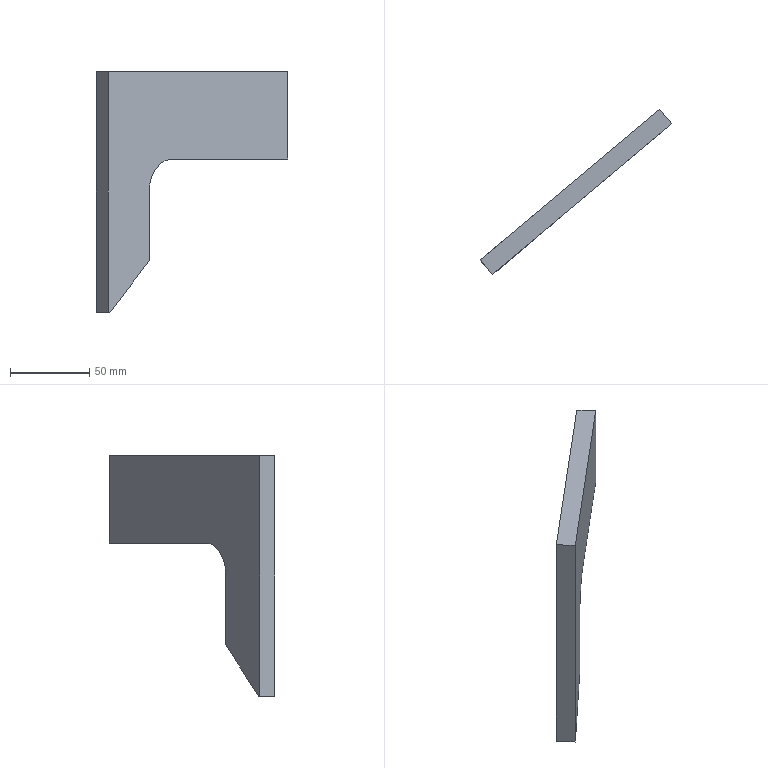Part | NX | features solid 2 | 1 solid | 10 faces | box 121.088 x 104.325 x 152 mm | volume 131882 mm3 | plane 9 | cylinder 1 | commonest cylinder face diameters 40 x1
STEP:
#1=CARTESIAN_POINT('',(765.225,419.33,-5.145));
#2=VERTEX_POINT('',#1);
#3=CARTESIAN_POINT('',(751.743,408.018,-25.));
#4=VERTEX_POINT('',#3);
#5=CARTESIAN_POINT('',(767.064,420.874,-25.));
#6=DIRECTION('',(0.6428,-0.766,0.));
#7=DIRECTION('',(0.766,0.6428,0.));
#8=AXIS2_PLACEMENT_3D('',#5,#6,#7);
#9=CIRCLE('',#8,20.);
#10=EDGE_CURVE('',#2,#4,#9,.T.);
#11=ORIENTED_EDGE('',*,*,#10,.F.);
#12=CARTESIAN_POINT('',(772.938,410.138,-5.145));
#13=VERTEX_POINT('',#12);
#14=CARTESIAN_POINT('',(772.938,410.138,-5.145));
#15=DIRECTION('',(-0.6428,0.766,0.));
#16=VECTOR('',#15,1000.);
#17=LINE('',#14,#16);
#18=EDGE_CURVE('',#13,#2,#17,.T.);
#19=ORIENTED_EDGE('',*,*,#18,.F.);
#20=CARTESIAN_POINT('',(759.457,398.826,-25.));
#21=VERTEX_POINT('',#20);
#22=CARTESIAN_POINT('',(774.777,411.681,-25.));
#23=DIRECTION('',(0.6428,-0.766,0.));
#24=DIRECTION('',(0.766,0.6428,0.));
#25=AXIS2_PLACEMENT_3D('',#22,#23,#24);
#26=CIRCLE('',#25,20.);
#27=EDGE_CURVE('',#13,#21,#26,.T.);
#28=ORIENTED_EDGE('',*,*,#27,.T.);
#29=CARTESIAN_POINT('',(759.457,398.826,-25.));
#30=DIRECTION('',(-0.6428,0.766,0.));
#31=VECTOR('',#30,1000.);
#32=LINE('',#29,#31);
#33=EDGE_CURVE('',#21,#4,#32,.T.);
#34=ORIENTED_EDGE('',*,*,#33,.T.);
#35=EDGE_LOOP('',(#11,#19,#28,#34));
#36=FACE_BOUND('',#35,.T.);
#37=CARTESIAN_POINT('',(774.777,411.681,-25.));
#38=DIRECTION('',(-0.6428,0.766,0.));
#39=DIRECTION('',(0.,0.,-1.));
#40=AXIS2_PLACEMENT_3D('',#37,#38,#39);
#41=CYLINDRICAL_SURFACE('',#40,20.);
#42=ADVANCED_FACE('',(#36),#41,.F.);
#43=CARTESIAN_POINT('',(839.225,481.424,-5.145));
#44=VERTEX_POINT('',#43);
#45=CARTESIAN_POINT('',(747.3,404.29,-5.145));
#46=DIRECTION('',(0.766,0.6428,0.));
#47=VECTOR('',#46,1000.);
#48=LINE('',#45,#47);
#49=EDGE_CURVE('',#2,#44,#48,.T.);
#50=ORIENTED_EDGE('',*,*,#49,.T.);
#51=CARTESIAN_POINT('',(846.939,472.232,-5.145));
#52=VERTEX_POINT('',#51);
#53=CARTESIAN_POINT('',(846.939,472.232,-5.145));
#54=DIRECTION('',(-0.6428,0.766,0.));
#55=VECTOR('',#54,1000.);
#56=LINE('',#53,#55);
#57=EDGE_CURVE('',#52,#44,#56,.T.);
#58=ORIENTED_EDGE('',*,*,#57,.F.);
#59=CARTESIAN_POINT('',(755.013,395.097,-5.145));
#60=DIRECTION('',(0.766,0.6428,0.));
#61=VECTOR('',#60,1000.);
#62=LINE('',#59,#61);
#63=EDGE_CURVE('',#13,#52,#62,.T.);
#64=ORIENTED_EDGE('',*,*,#63,.F.);
#65=ORIENTED_EDGE('',*,*,#18,.T.);
#66=EDGE_LOOP('',(#50,#58,#64,#65));
#67=FACE_BOUND('',#66,.T.);
#68=CARTESIAN_POINT('',(755.013,395.097,-5.145));
#69=DIRECTION('',(0.,0.,1.));
#70=DIRECTION('',(-0.766,-0.6428,0.));
#71=AXIS2_PLACEMENT_3D('',#68,#69,#70);
#72=PLANE('',#71);
#73=ADVANCED_FACE('',(#67),#72,.F.);
#74=CARTESIAN_POINT('',(839.225,481.424,50.));
#75=VERTEX_POINT('',#74);
#76=CARTESIAN_POINT('',(839.225,481.424,-5.145));
#77=DIRECTION('',(0.,0.,1.));
#78=VECTOR('',#77,1000.);
#79=LINE('',#76,#78);
#80=EDGE_CURVE('',#44,#75,#79,.T.);
#81=ORIENTED_EDGE('',*,*,#80,.T.);
#82=CARTESIAN_POINT('',(846.939,472.232,50.));
#83=VERTEX_POINT('',#82);
#84=CARTESIAN_POINT('',(846.939,472.232,50.));
#85=DIRECTION('',(-0.6428,0.766,0.));
#86=VECTOR('',#85,1000.);
#87=LINE('',#84,#86);
#88=EDGE_CURVE('',#83,#75,#87,.T.);
#89=ORIENTED_EDGE('',*,*,#88,.F.);
#90=CARTESIAN_POINT('',(846.939,472.232,-5.145));
#91=DIRECTION('',(0.,0.,1.));
#92=VECTOR('',#91,1000.);
#93=LINE('',#90,#92);
#94=EDGE_CURVE('',#52,#83,#93,.T.);
#95=ORIENTED_EDGE('',*,*,#94,.F.);
#96=ORIENTED_EDGE('',*,*,#57,.T.);
#97=EDGE_LOOP('',(#81,#89,#95,#96));
#98=FACE_BOUND('',#97,.T.);
#99=CARTESIAN_POINT('',(846.939,472.232,-5.145));
#100=DIRECTION('',(-0.766,-0.6428,0.));
#101=DIRECTION('',(0.,0.,-1.));
#102=AXIS2_PLACEMENT_3D('',#99,#100,#101);
#103=PLANE('',#102);
#104=ADVANCED_FACE('',(#98),#103,.F.);
#105=CARTESIAN_POINT('',(725.851,386.292,-102.));
#106=VERTEX_POINT('',#105);
#107=CARTESIAN_POINT('',(725.851,386.292,50.));
#108=VERTEX_POINT('',#107);
#109=CARTESIAN_POINT('',(725.851,386.292,-102.));
#110=DIRECTION('',(0.,0.,1.));
#111=VECTOR('',#110,1000.);
#112=LINE('',#109,#111);
#113=EDGE_CURVE('',#106,#108,#112,.T.);
#114=ORIENTED_EDGE('',*,*,#113,.F.);
#115=CARTESIAN_POINT('',(733.564,377.099,-102.));
#116=VERTEX_POINT('',#115);
#117=CARTESIAN_POINT('',(733.564,377.099,-102.));
#118=DIRECTION('',(-0.6428,0.766,0.));
#119=VECTOR('',#118,1000.);
#120=LINE('',#117,#119);
#121=EDGE_CURVE('',#116,#106,#120,.T.);
#122=ORIENTED_EDGE('',*,*,#121,.F.);
#123=CARTESIAN_POINT('',(733.564,377.099,50.));
#124=VERTEX_POINT('',#123);
#125=CARTESIAN_POINT('',(733.564,377.099,-102.));
#126=DIRECTION('',(0.,0.,1.));
#127=VECTOR('',#126,1000.);
#128=LINE('',#125,#127);
#129=EDGE_CURVE('',#116,#124,#128,.T.);
#130=ORIENTED_EDGE('',*,*,#129,.T.);
#131=CARTESIAN_POINT('',(733.564,377.099,50.));
#132=DIRECTION('',(-0.6428,0.766,0.));
#133=VECTOR('',#132,1000.);
#134=LINE('',#131,#133);
#135=EDGE_CURVE('',#124,#108,#134,.T.);
#136=ORIENTED_EDGE('',*,*,#135,.T.);
#137=EDGE_LOOP('',(#114,#122,#130,#136));
#138=FACE_BOUND('',#137,.T.);
#139=CARTESIAN_POINT('',(733.564,377.099,-102.));
#140=DIRECTION('',(-0.766,-0.6428,0.));
#141=DIRECTION('',(0.,0.,-1.));
#142=AXIS2_PLACEMENT_3D('',#139,#140,#141);
#143=PLANE('',#142);
#144=ADVANCED_FACE('',(#138),#143,.T.);
#145=CARTESIAN_POINT('',(726.847,387.128,-102.));
#146=VERTEX_POINT('',#145);
#147=CARTESIAN_POINT('',(726.847,387.128,-102.));
#148=DIRECTION('',(-0.766,-0.6428,0.));
#149=VECTOR('',#148,1000.);
#150=LINE('',#147,#149);
#151=EDGE_CURVE('',#146,#106,#150,.T.);
#152=ORIENTED_EDGE('',*,*,#151,.F.);
#153=CARTESIAN_POINT('',(734.56,377.935,-102.));
#154=VERTEX_POINT('',#153);
#155=CARTESIAN_POINT('',(734.56,377.935,-102.));
#156=DIRECTION('',(-0.6428,0.766,0.));
#157=VECTOR('',#156,1000.);
#158=LINE('',#155,#157);
#159=EDGE_CURVE('',#154,#146,#158,.T.);
#160=ORIENTED_EDGE('',*,*,#159,.F.);
#161=CARTESIAN_POINT('',(734.56,377.935,-102.));
#162=DIRECTION('',(-0.766,-0.6428,0.));
#163=VECTOR('',#162,1000.);
#164=LINE('',#161,#163);
#165=EDGE_CURVE('',#154,#116,#164,.T.);
#166=ORIENTED_EDGE('',*,*,#165,.T.);
#167=ORIENTED_EDGE('',*,*,#121,.T.);
#168=EDGE_LOOP('',(#152,#160,#166,#167));
#169=FACE_BOUND('',#168,.T.);
#170=CARTESIAN_POINT('',(734.56,377.935,-102.));
#171=DIRECTION('',(0.,0.,-1.));
#172=DIRECTION('',(0.766,0.6428,0.));
#173=AXIS2_PLACEMENT_3D('',#170,#171,#172);
#174=PLANE('',#173);
#175=ADVANCED_FACE('',(#169),#174,.T.);
#176=CARTESIAN_POINT('',(751.743,408.018,-69.5));
#177=VERTEX_POINT('',#176);
#178=CARTESIAN_POINT('',(726.847,387.128,-102.));
#179=DIRECTION('',(0.5417,0.4545,0.7071));
#180=VECTOR('',#179,1000.);
#181=LINE('',#178,#180);
#182=EDGE_CURVE('',#146,#177,#181,.T.);
#183=ORIENTED_EDGE('',*,*,#182,.T.);
#184=CARTESIAN_POINT('',(759.457,398.826,-69.5));
#185=VERTEX_POINT('',#184);
#186=CARTESIAN_POINT('',(759.457,398.826,-69.5));
#187=DIRECTION('',(-0.6428,0.766,0.));
#188=VECTOR('',#187,1000.);
#189=LINE('',#186,#188);
#190=EDGE_CURVE('',#185,#177,#189,.T.);
#191=ORIENTED_EDGE('',*,*,#190,.F.);
#192=CARTESIAN_POINT('',(734.56,377.935,-102.));
#193=DIRECTION('',(0.5417,0.4545,0.7071));
#194=VECTOR('',#193,1000.);
#195=LINE('',#192,#194);
#196=EDGE_CURVE('',#154,#185,#195,.T.);
#197=ORIENTED_EDGE('',*,*,#196,.F.);
#198=ORIENTED_EDGE('',*,*,#159,.T.);
#199=EDGE_LOOP('',(#183,#191,#197,#198));
#200=FACE_BOUND('',#199,.T.);
#201=CARTESIAN_POINT('',(734.56,377.935,-102.));
#202=DIRECTION('',(-0.5417,-0.4545,0.7071));
#203=DIRECTION('',(-0.5417,-0.4545,-0.7071));
#204=AXIS2_PLACEMENT_3D('',#201,#202,#203);
#205=PLANE('',#204);
#206=ADVANCED_FACE('',(#200),#205,.F.);
#207=CARTESIAN_POINT('',(751.743,408.018,-69.5));
#208=DIRECTION('',(0.,0.,1.));
#209=VECTOR('',#208,1000.);
#210=LINE('',#207,#209);
#211=EDGE_CURVE('',#177,#4,#210,.T.);
#212=ORIENTED_EDGE('',*,*,#211,.T.);
#213=ORIENTED_EDGE('',*,*,#33,.F.);
#214=CARTESIAN_POINT('',(759.457,398.826,-69.5));
#215=DIRECTION('',(0.,0.,1.));
#216=VECTOR('',#215,1000.);
#217=LINE('',#214,#216);
#218=EDGE_CURVE('',#185,#21,#217,.T.);
#219=ORIENTED_EDGE('',*,*,#218,.F.);
#220=ORIENTED_EDGE('',*,*,#190,.T.);
#221=EDGE_LOOP('',(#212,#213,#219,#220));
#222=FACE_BOUND('',#221,.T.);
#223=CARTESIAN_POINT('',(759.457,398.826,-69.5));
#224=DIRECTION('',(-0.766,-0.6428,0.));
#225=DIRECTION('',(0.,0.,-1.));
#226=AXIS2_PLACEMENT_3D('',#223,#224,#225);
#227=PLANE('',#226);
#228=ADVANCED_FACE('',(#222),#227,.F.);
#229=ORIENTED_EDGE('',*,*,#27,.F.);
#230=ORIENTED_EDGE('',*,*,#63,.T.);
#231=ORIENTED_EDGE('',*,*,#94,.T.);
#232=CARTESIAN_POINT('',(728.202,372.6,50.));
#233=DIRECTION('',(0.766,0.6428,0.));
#234=VECTOR('',#233,1000.);
#235=LINE('',#232,#234);
#236=EDGE_CURVE('',#124,#83,#235,.T.);
#237=ORIENTED_EDGE('',*,*,#236,.F.);
#238=ORIENTED_EDGE('',*,*,#129,.F.);
#239=ORIENTED_EDGE('',*,*,#165,.F.);
#240=ORIENTED_EDGE('',*,*,#196,.T.);
#241=ORIENTED_EDGE('',*,*,#218,.T.);
#242=EDGE_LOOP('',(#229,#230,#231,#237,#238,#239,#240,#241));
#243=FACE_BOUND('',#242,.T.);
#244=CARTESIAN_POINT('',(755.521,395.523,-33.617));
#245=DIRECTION('',(0.6428,-0.766,0.));
#246=DIRECTION('',(0.,0.,1.));
#247=AXIS2_PLACEMENT_3D('',#244,#245,#246);
#248=PLANE('',#247);
#249=ADVANCED_FACE('',(#243),#248,.T.);
#250=ORIENTED_EDGE('',*,*,#10,.T.);
#251=ORIENTED_EDGE('',*,*,#211,.F.);
#252=ORIENTED_EDGE('',*,*,#182,.F.);
#253=ORIENTED_EDGE('',*,*,#151,.T.);
#254=ORIENTED_EDGE('',*,*,#113,.T.);
#255=CARTESIAN_POINT('',(720.488,381.792,50.));
#256=DIRECTION('',(0.766,0.6428,0.));
#257=VECTOR('',#256,1000.);
#258=LINE('',#255,#257);
#259=EDGE_CURVE('',#108,#75,#258,.T.);
#260=ORIENTED_EDGE('',*,*,#259,.T.);
#261=ORIENTED_EDGE('',*,*,#80,.F.);
#262=ORIENTED_EDGE('',*,*,#49,.F.);
#263=EDGE_LOOP('',(#250,#251,#252,#253,#254,#260,#261,#262));
#264=FACE_BOUND('',#263,.T.);
#265=CARTESIAN_POINT('',(747.807,404.716,-33.617));
#266=DIRECTION('',(0.6428,-0.766,0.));
#267=DIRECTION('',(0.,0.,1.));
#268=AXIS2_PLACEMENT_3D('',#265,#266,#267);
#269=PLANE('',#268);
#270=ADVANCED_FACE('',(#264),#269,.F.);
#271=ORIENTED_EDGE('',*,*,#259,.F.);
#272=ORIENTED_EDGE('',*,*,#135,.F.);
#273=ORIENTED_EDGE('',*,*,#236,.T.);
#274=ORIENTED_EDGE('',*,*,#88,.T.);
#275=EDGE_LOOP('',(#271,#272,#273,#274));
#276=FACE_BOUND('',#275,.T.);
#277=CARTESIAN_POINT('',(728.202,372.6,50.));
#278=DIRECTION('',(0.,0.,1.));
#279=DIRECTION('',(-0.766,-0.6428,0.));
#280=AXIS2_PLACEMENT_3D('',#277,#278,#279);
#281=PLANE('',#280);
#282=ADVANCED_FACE('',(#276),#281,.T.);
#283=CLOSED_SHELL('',(#42,#73,#104,#144,#175,#206,#228,#249,#270,#282));
#284=MANIFOLD_SOLID_BREP('',#283);
#285=(LENGTH_UNIT()NAMED_UNIT(*)SI_UNIT(.MILLI.,.METRE.));
#286=UNCERTAINTY_MEASURE_WITH_UNIT(LENGTH_MEASURE(0.00001),#285,'','');
#287=(NAMED_UNIT(*)PLANE_ANGLE_UNIT()SI_UNIT($,.RADIAN.));
#288=(NAMED_UNIT(*)SI_UNIT($,.STERADIAN.)SOLID_ANGLE_UNIT());
#289=(GEOMETRIC_REPRESENTATION_CONTEXT(3)GLOBAL_UNCERTAINTY_ASSIGNED_CONTEXT((#286))GLOBAL_UNIT_ASSIGNED_CONTEXT((#285,#287,#288))REPRESENTATION_CONTEXT('',''));
#290=ADVANCED_BREP_SHAPE_REPRESENTATION('',(#284),#289);